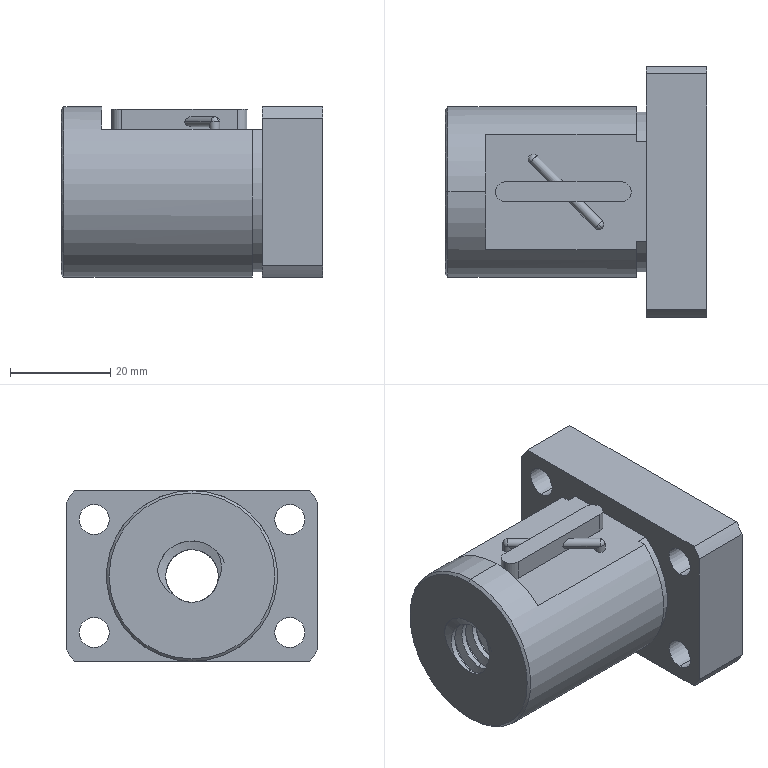Part | SolidWorks | features ICE 8, Revolution 4, RefAxis 3, RevCut 2, 3DProfileFeature 1, Helix 1, SweepCut 1 | 2 solids | 116 faces | box 52 x 50 x 34 mm | volume 45697 mm3 | cylinder 82 | plane 19 | spline 8 | cone 4 | sphere 3 | commonest cylinder face diameters 10.5 x43 2 x8 6 x8 9.5 x8 4.917 x5 58 x4